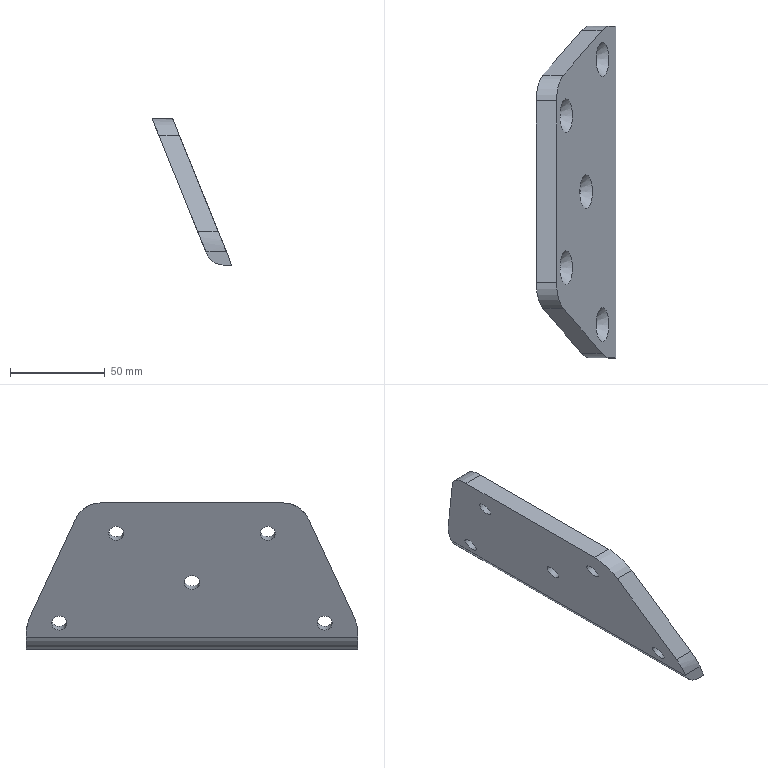Part | STEP file | solid 37 | 1 solid | 23 faces | box 41.968 x 175 x 77.179 mm | volume 118228 mm3 | cylinder 10 | plane 8 | cone 5 | commonest cylinder face diameters 8 x5 30 x2 51 x2 20 x1